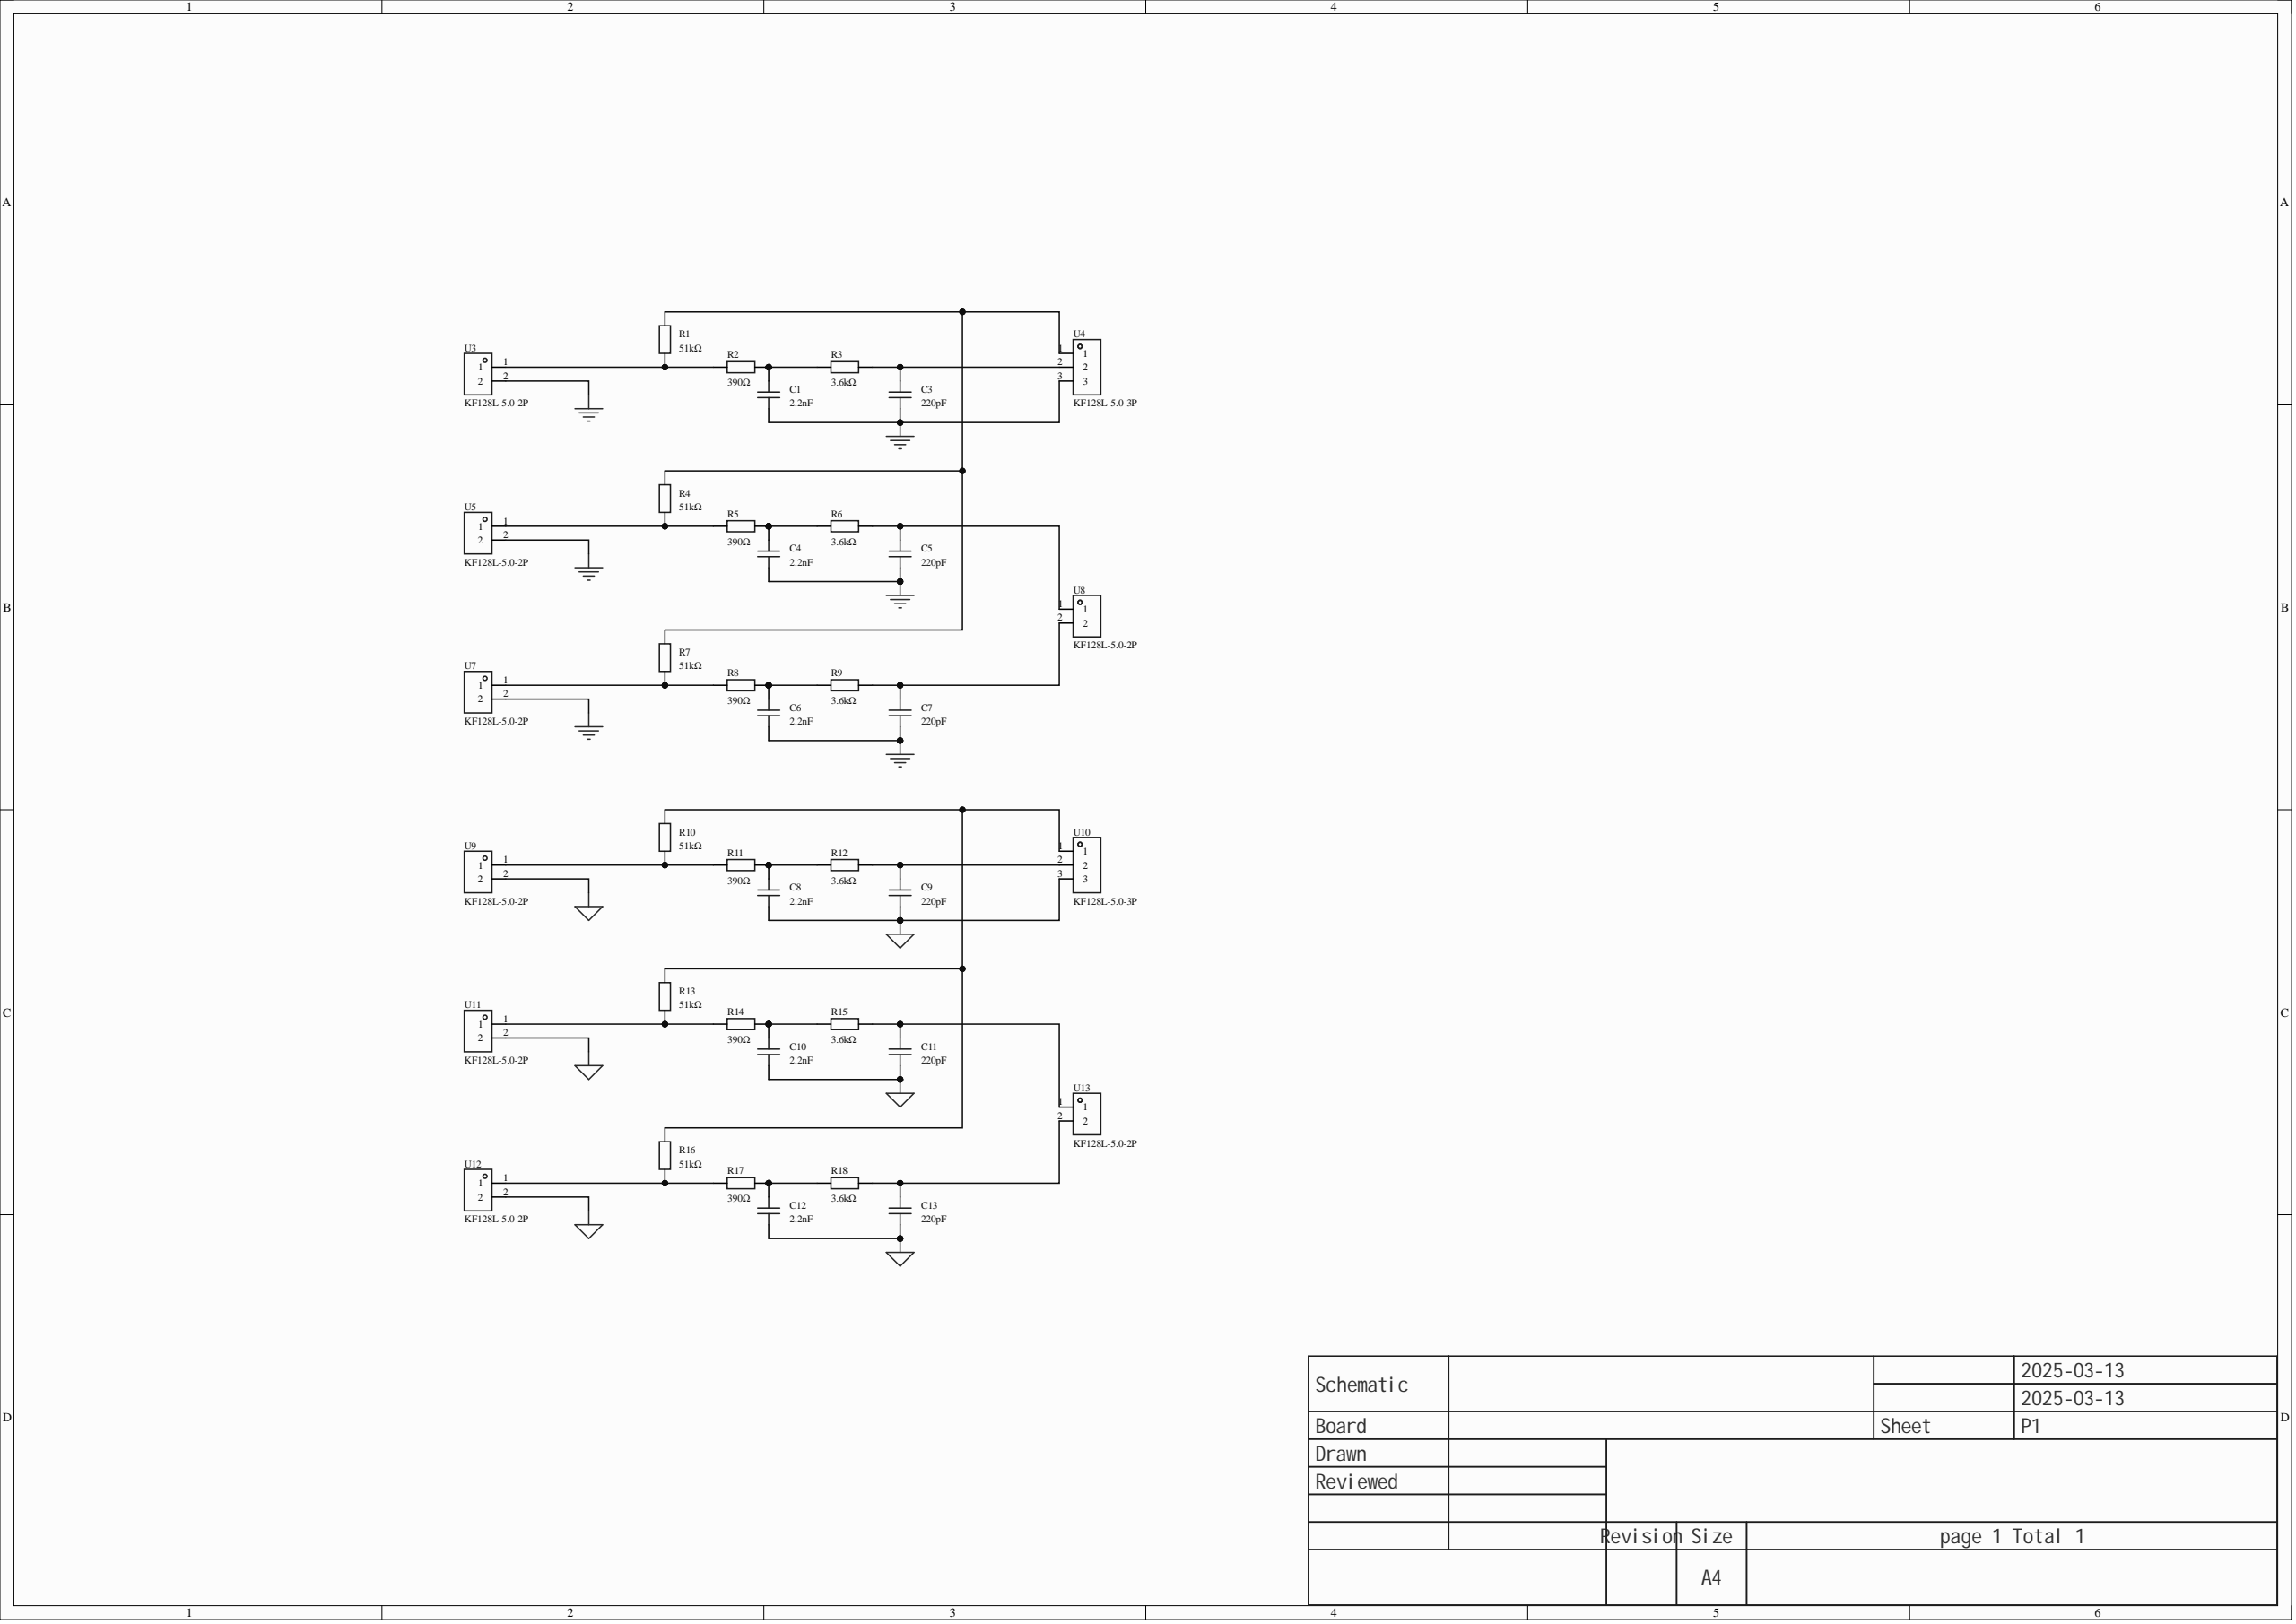Circuit board | Altium Designer | 40 parts | 22 nets
Bill of materials:
Comment,Description,Designator,Footprint,LibRef,Quantity
"2.2nF","component DE2E3KY222MA3BU02F capacitance:2.2nF;tolerance:±20%;voltage(AC):300V;class:X1,Y2;","C1, C4, C6, C8, C10, C12","CAP-TH_L8.0-W5.0-P7.50-D1.0","DE2E3KY222MA3BU02F","6"
"220pF","component KP1830122633 compo capacitance:220pF;tolerance:±2.5%;rated voltage:630V; 250V;operating temperature:-55℃~+100℃;","C3, C5, C7, C9, C11, C13","CAP-TH_L7.2-W4.5-P5.00-D0.5","KP1830122633","6"
"51kΩ","","R1, R4, R7, R10, R13, R16","Res_1/4W","Res_AXIAL-1/4W","6"
"390Ω","","R2, R5, R8, R11, R14, R17","Res_1/4W","Res_AXIAL-1/4W","6"
"3.6kΩ","","R3, R6, R9, R12, R15, R18","Res_1/4W","Res_AXIAL-1/4W","6"
"KF128L-5.0-2P","","U3, U5, U7, U8, U9, U11, U12, U13","CONN-TH_P5.00_KF128L-5.0-2P","KF128L-5.0-2P","8"
"KF128L-5.0-3P","","U4, U10","CONN-TH_3P-P5.00_KF128L-5.0-3P","KF128L-5.0-3P","2"
Netlist (Protel format):
[
C1
CAP-TH_L8.0-W5.0-P7.50-D1.0
2.2nF



]
[
C3
CAP-TH_L7.2-W4.5-P5.00-D0.5
220pF



]
[
C4
CAP-TH_L8.0-W5.0-P7.50-D1.0
2.2nF



]
[
C5
CAP-TH_L7.2-W4.5-P5.00-D0.5
220pF



]
[
C6
CAP-TH_L8.0-W5.0-P7.50-D1.0
2.2nF



]
[
C7
CAP-TH_L7.2-W4.5-P5.00-D0.5
220pF



]
[
C8
CAP-TH_L8.0-W5.0-P7.50-D1.0
2.2nF



]
[
C9
CAP-TH_L7.2-W4.5-P5.00-D0.5
220pF



]
[
C10
CAP-TH_L8.0-W5.0-P7.50-D1.0
2.2nF



]
[
C11
CAP-TH_L7.2-W4.5-P5.00-D0.5
220pF



]
[
C12
CAP-TH_L8.0-W5.0-P7.50-D1.0
2.2nF



]
[
C13
CAP-TH_L7.2-W4.5-P5.00-D0.5
220pF



]
[
R1
Res_1/4W
51kΩ



]
[
R2
Res_1/4W
390Ω



]
[
R3
Res_1/4W
3.6kΩ



]
[
R4
Res_1/4W
51kΩ



]
[
R5
Res_1/4W
390Ω



]
[
R6
Res_1/4W
3.6kΩ



]
[
R7
Res_1/4W
51kΩ



]
[
R8
Res_1/4W
390Ω



]
[
R9
Res_1/4W
3.6kΩ



]
[
R10
Res_1/4W
51kΩ



]
[
R11
Res_1/4W
390Ω



]
[
R12
Res_1/4W
3.6kΩ



]
[
R13
Res_1/4W
51kΩ



]
[
R14
Res_1/4W
390Ω



]
[
R15
Res_1/4W
3.6kΩ



]
[
R16
Res_1/4W
51kΩ



]
[
R17
Res_1/4W
390Ω



]
[
R18
Res_1/4W
3.6kΩ



]
[
U3
CONN-TH_P5.00_KF128L-5.0-2P
KF128L-5.0-2P



]
[
U4
CONN-TH_3P-P5.00_KF128L-5.0-3P
KF128L-5.0-3P



]
[
U5
CONN-TH_P5.00_KF128L-5.0-2P
KF128L-5.0-2P



]
[
U7
CONN-TH_P5.00_KF128L-5.0-2P
KF128L-5.0-2P



]
[
U8
CONN-TH_P5.00_KF128L-5.0-2P
KF128L-5.0-2P



]
[
U9
CONN-TH_P5.00_KF128L-5.0-2P
KF128L-5.0-2P



]
[
U10
CONN-TH_3P-P5.00_KF128L-5.0-3P
KF128L-5.0-3P



]
[
U11
CONN-TH_P5.00_KF128L-5.0-2P
KF128L-5.0-2P



]
[
U12
CONN-TH_P5.00_KF128L-5.0-2P
KF128L-5.0-2P



]
[
U13
CONN-TH_P5.00_KF128L-5.0-2P
KF128L-5.0-2P



]
(
NetR16_1
R16-1
R17-2
U12-1
)
(
NetR13_1
R13-1
R14-2
U11-1
)
(
NetR10_2
R10-2
R13-2
R16-2
U10-1
)
(
NetR10_1
R10-1
R11-2
U9-1
)
(
NetR7_1
R7-1
R8-2
U7-1
)
(
NetR4_1
R4-1
R5-2
U5-1
)
(
NetR1_2
R1-2
R4-2
R7-2
U4-1
)
(
NetR1_1
R1-1
R2-2
U3-1
)
(
NetC13_2
C13-2
R18-1
U13-2
)
(
NetC12_2
C12-2
R17-1
R18-2
)
(
NetC11_2
C11-2
R15-1
U13-1
)
(
NetC10_2
C10-2
R14-1
R15-2
)
(
NetC9_2
C9-2
R12-1
U10-2
)
(
NetC8_2
C8-2
R11-1
R12-2
)
(
NetC7_2
C7-2
R9-1
U8-2
)
(
NetC6_2
C6-2
R8-1
R9-2
)
(
NetC5_2
C5-2
R6-1
U8-1
)
(
NetC4_2
C4-2
R5-1
R6-2
)
(
NetC3_2
C3-2
R3-1
U4-2
)
(
NetC1_2
C1-2
R2-1
R3-2
)
(
GND
C1-1
C3-1
C4-1
C5-1
C6-1
C7-1
U3-2
U4-3
U5-2
U7-2
)
(
AGND
C8-1
C9-1
C10-1
C11-1
C12-1
C13-1
U9-2
U10-3
U11-2
U12-2
)